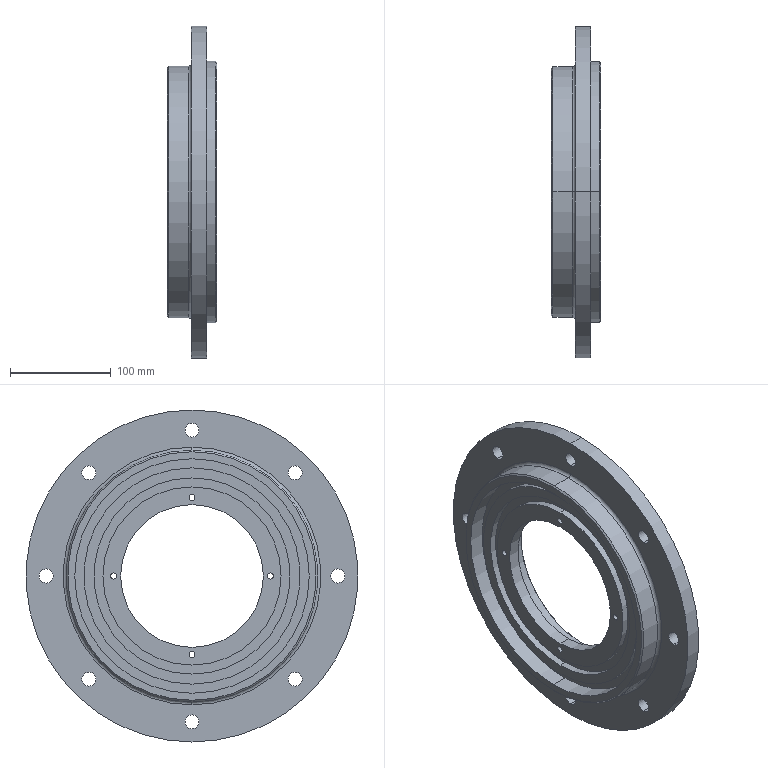Part | STEP file | Through-hole cover | 1 solid | 62 faces | box 49 x 330 x 330 mm | volume 1508672 mm3 | cylinder 42 | plane 10 | cone 8 | torus 2 | commonest cylinder face diameters 14 x16 6 x8 142 x2 170 x2 177 x2 195 x2